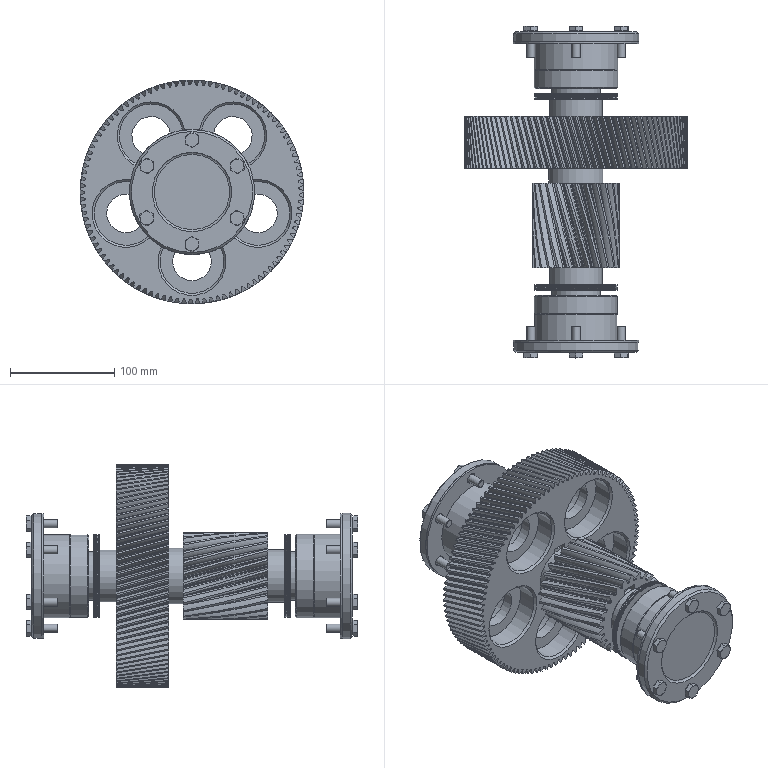Part | NX | 45 solids | 1268 faces | box 214.08 x 317.8 x 214.08 mm | volume 2085150 mm3 | spline 630 | cylinder 228 | plane 190 | cone 182 | torus 20 | sphere 18 | commonest cylinder face diameters 205.08 x101 70.33 x25 9 x24 7.76 x12 11.63 x12 61 x10